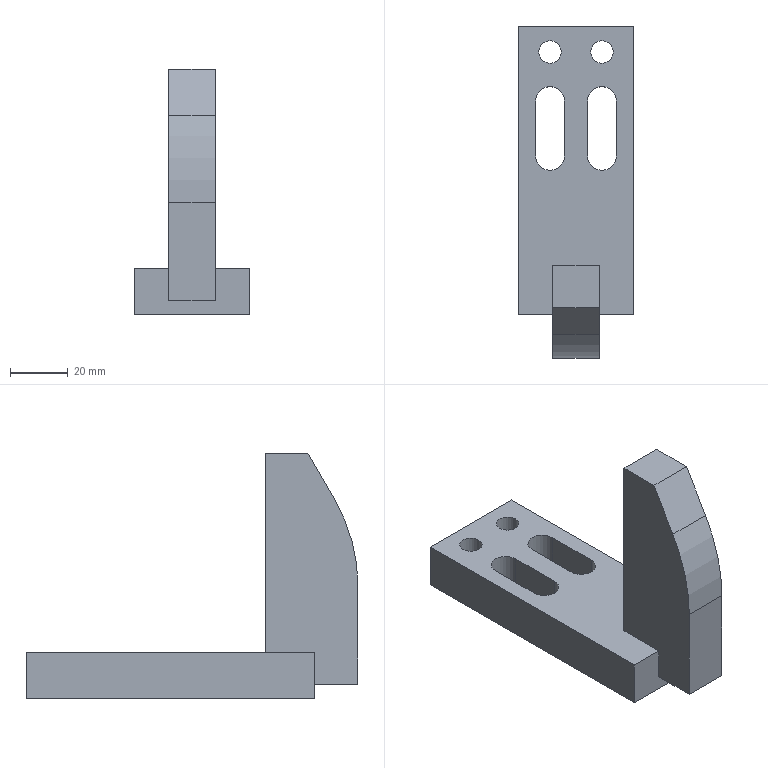Part | NX | features solid 2 | 1 solid | 24 faces | box 40 x 115 x 85 mm | volume 87334 mm3 | plane 17 | cylinder 7 | commonest cylinder face diameters 10 x4 7.8 x2 120 x1
STEP:
#1=CARTESIAN_POINT('',(797.6,496.,-19.));
#2=VERTEX_POINT('',#1);
#3=CARTESIAN_POINT('',(801.5,496.,-19.));
#4=DIRECTION('',(0.,0.,-1.));
#5=DIRECTION('',(-1.,0.,0.));
#6=AXIS2_PLACEMENT_3D('',#3,#4,#5);
#7=CIRCLE('',#6,3.9);
#8=EDGE_CURVE('',#2,#2,#7,.T.);
#9=ORIENTED_EDGE('',*,*,#8,.T.);
#10=EDGE_LOOP('',(#9));
#11=FACE_BOUND('',#10,.T.);
#12=CARTESIAN_POINT('',(806.5,460.,-19.));
#13=VERTEX_POINT('',#12);
#14=CARTESIAN_POINT('',(796.5,460.,-19.));
#15=VERTEX_POINT('',#14);
#16=CARTESIAN_POINT('',(801.5,460.,-19.));
#17=DIRECTION('',(0.,0.,-1.));
#18=DIRECTION('',(-1.,0.,0.));
#19=AXIS2_PLACEMENT_3D('',#16,#17,#18);
#20=CIRCLE('',#19,5.);
#21=EDGE_CURVE('',#13,#15,#20,.T.);
#22=ORIENTED_EDGE('',*,*,#21,.T.);
#23=CARTESIAN_POINT('',(796.5,479.,-19.));
#24=VERTEX_POINT('',#23);
#25=CARTESIAN_POINT('',(796.5,535.,-19.));
#26=DIRECTION('',(0.,-1.,0.));
#27=VECTOR('',#26,1000.);
#28=LINE('',#25,#27);
#29=EDGE_CURVE('',#24,#15,#28,.T.);
#30=ORIENTED_EDGE('',*,*,#29,.F.);
#31=CARTESIAN_POINT('',(806.5,479.,-19.));
#32=VERTEX_POINT('',#31);
#33=CARTESIAN_POINT('',(801.5,479.,-19.));
#34=DIRECTION('',(0.,0.,-1.));
#35=DIRECTION('',(-1.,0.,0.));
#36=AXIS2_PLACEMENT_3D('',#33,#34,#35);
#37=CIRCLE('',#36,5.);
#38=EDGE_CURVE('',#24,#32,#37,.T.);
#39=ORIENTED_EDGE('',*,*,#38,.T.);
#40=CARTESIAN_POINT('',(806.5,535.,-19.));
#41=DIRECTION('',(0.,1.,0.));
#42=VECTOR('',#41,1000.);
#43=LINE('',#40,#42);
#44=EDGE_CURVE('',#13,#32,#43,.T.);
#45=ORIENTED_EDGE('',*,*,#44,.F.);
#46=EDGE_LOOP('',(#22,#30,#39,#45));
#47=FACE_BOUND('',#46,.T.);
#48=CARTESIAN_POINT('',(779.6,496.,-19.));
#49=VERTEX_POINT('',#48);
#50=CARTESIAN_POINT('',(783.5,496.,-19.));
#51=DIRECTION('',(0.,0.,-1.));
#52=DIRECTION('',(-1.,0.,0.));
#53=AXIS2_PLACEMENT_3D('',#50,#51,#52);
#54=CIRCLE('',#53,3.9);
#55=EDGE_CURVE('',#49,#49,#54,.T.);
#56=ORIENTED_EDGE('',*,*,#55,.T.);
#57=EDGE_LOOP('',(#56));
#58=FACE_BOUND('',#57,.T.);
#59=CARTESIAN_POINT('',(812.5,405.,-19.));
#60=VERTEX_POINT('',#59);
#61=CARTESIAN_POINT('',(800.5,405.,-19.));
#62=VERTEX_POINT('',#61);
#63=CARTESIAN_POINT('',(804.5,405.,-19.));
#64=DIRECTION('',(-1.,0.,0.));
#65=VECTOR('',#64,1000.);
#66=LINE('',#63,#65);
#67=EDGE_CURVE('',#60,#62,#66,.T.);
#68=ORIENTED_EDGE('',*,*,#67,.F.);
#69=CARTESIAN_POINT('',(812.5,505.,-19.));
#70=VERTEX_POINT('',#69);
#71=CARTESIAN_POINT('',(812.5,505.,-19.));
#72=DIRECTION('',(0.,-1.,0.));
#73=VECTOR('',#72,1000.);
#74=LINE('',#71,#73);
#75=EDGE_CURVE('',#70,#60,#74,.T.);
#76=ORIENTED_EDGE('',*,*,#75,.F.);
#77=CARTESIAN_POINT('',(772.5,505.,-19.));
#78=VERTEX_POINT('',#77);
#79=CARTESIAN_POINT('',(804.5,505.,-19.));
#80=DIRECTION('',(1.,0.,0.));
#81=VECTOR('',#80,1000.);
#82=LINE('',#79,#81);
#83=EDGE_CURVE('',#78,#70,#82,.T.);
#84=ORIENTED_EDGE('',*,*,#83,.F.);
#85=CARTESIAN_POINT('',(772.5,405.,-19.));
#86=VERTEX_POINT('',#85);
#87=CARTESIAN_POINT('',(772.5,405.,-19.));
#88=DIRECTION('',(0.,1.,0.));
#89=VECTOR('',#88,1000.);
#90=LINE('',#87,#89);
#91=EDGE_CURVE('',#86,#78,#90,.T.);
#92=ORIENTED_EDGE('',*,*,#91,.F.);
#93=CARTESIAN_POINT('',(784.5,405.,-19.));
#94=VERTEX_POINT('',#93);
#95=CARTESIAN_POINT('',(804.5,405.,-19.));
#96=DIRECTION('',(-1.,0.,0.));
#97=VECTOR('',#96,1000.);
#98=LINE('',#95,#97);
#99=EDGE_CURVE('',#94,#86,#98,.T.);
#100=ORIENTED_EDGE('',*,*,#99,.F.);
#101=CARTESIAN_POINT('',(784.5,422.,-19.));
#102=VERTEX_POINT('',#101);
#103=CARTESIAN_POINT('',(784.5,505.,-19.));
#104=DIRECTION('',(0.,1.,0.));
#105=VECTOR('',#104,1000.);
#106=LINE('',#103,#105);
#107=EDGE_CURVE('',#94,#102,#106,.T.);
#108=ORIENTED_EDGE('',*,*,#107,.T.);
#109=CARTESIAN_POINT('',(800.5,422.,-19.));
#110=VERTEX_POINT('',#109);
#111=CARTESIAN_POINT('',(804.5,422.,-19.));
#112=DIRECTION('',(1.,0.,0.));
#113=VECTOR('',#112,1000.);
#114=LINE('',#111,#113);
#115=EDGE_CURVE('',#102,#110,#114,.T.);
#116=ORIENTED_EDGE('',*,*,#115,.T.);
#117=CARTESIAN_POINT('',(800.5,505.,-19.));
#118=DIRECTION('',(0.,1.,0.));
#119=VECTOR('',#118,1000.);
#120=LINE('',#117,#119);
#121=EDGE_CURVE('',#62,#110,#120,.T.);
#122=ORIENTED_EDGE('',*,*,#121,.F.);
#123=EDGE_LOOP('',(#68,#76,#84,#92,#100,#108,#116,#122));
#124=FACE_BOUND('',#123,.T.);
#125=CARTESIAN_POINT('',(778.5,479.,-19.));
#126=VERTEX_POINT('',#125);
#127=CARTESIAN_POINT('',(788.5,479.,-19.));
#128=VERTEX_POINT('',#127);
#129=CARTESIAN_POINT('',(783.5,479.,-19.));
#130=DIRECTION('',(0.,0.,-1.));
#131=DIRECTION('',(-1.,0.,0.));
#132=AXIS2_PLACEMENT_3D('',#129,#130,#131);
#133=CIRCLE('',#132,5.);
#134=EDGE_CURVE('',#126,#128,#133,.T.);
#135=ORIENTED_EDGE('',*,*,#134,.T.);
#136=CARTESIAN_POINT('',(788.5,460.,-19.));
#137=VERTEX_POINT('',#136);
#138=CARTESIAN_POINT('',(788.5,535.,-19.));
#139=DIRECTION('',(0.,1.,0.));
#140=VECTOR('',#139,1000.);
#141=LINE('',#138,#140);
#142=EDGE_CURVE('',#137,#128,#141,.T.);
#143=ORIENTED_EDGE('',*,*,#142,.F.);
#144=CARTESIAN_POINT('',(778.5,460.,-19.));
#145=VERTEX_POINT('',#144);
#146=CARTESIAN_POINT('',(783.5,460.,-19.));
#147=DIRECTION('',(0.,0.,-1.));
#148=DIRECTION('',(-1.,0.,0.));
#149=AXIS2_PLACEMENT_3D('',#146,#147,#148);
#150=CIRCLE('',#149,5.);
#151=EDGE_CURVE('',#137,#145,#150,.T.);
#152=ORIENTED_EDGE('',*,*,#151,.T.);
#153=CARTESIAN_POINT('',(778.5,535.,-19.));
#154=DIRECTION('',(0.,-1.,0.));
#155=VECTOR('',#154,1000.);
#156=LINE('',#153,#155);
#157=EDGE_CURVE('',#126,#145,#156,.T.);
#158=ORIENTED_EDGE('',*,*,#157,.F.);
#159=EDGE_LOOP('',(#135,#143,#152,#158));
#160=FACE_BOUND('',#159,.T.);
#161=CARTESIAN_POINT('',(804.5,505.,-19.));
#162=DIRECTION('',(0.,0.,1.));
#163=DIRECTION('',(0.,1.,0.));
#164=AXIS2_PLACEMENT_3D('',#161,#162,#163);
#165=PLANE('',#164);
#166=ADVANCED_FACE('',(#11,#47,#58,#124,#160),#165,.T.);
#167=CARTESIAN_POINT('',(797.6,496.,-35.));
#168=VERTEX_POINT('',#167);
#169=CARTESIAN_POINT('',(801.5,496.,-35.));
#170=DIRECTION('',(0.,0.,-1.));
#171=DIRECTION('',(-1.,0.,0.));
#172=AXIS2_PLACEMENT_3D('',#169,#170,#171);
#173=CIRCLE('',#172,3.9);
#174=EDGE_CURVE('',#168,#168,#173,.T.);
#175=ORIENTED_EDGE('',*,*,#174,.F.);
#176=EDGE_LOOP('',(#175));
#177=FACE_BOUND('',#176,.T.);
#178=CARTESIAN_POINT('',(806.5,460.,-35.));
#179=VERTEX_POINT('',#178);
#180=CARTESIAN_POINT('',(806.5,479.,-35.));
#181=VERTEX_POINT('',#180);
#182=CARTESIAN_POINT('',(806.5,535.,-35.));
#183=DIRECTION('',(0.,1.,0.));
#184=VECTOR('',#183,1000.);
#185=LINE('',#182,#184);
#186=EDGE_CURVE('',#179,#181,#185,.T.);
#187=ORIENTED_EDGE('',*,*,#186,.T.);
#188=CARTESIAN_POINT('',(796.5,479.,-35.));
#189=VERTEX_POINT('',#188);
#190=CARTESIAN_POINT('',(801.5,479.,-35.));
#191=DIRECTION('',(0.,0.,-1.));
#192=DIRECTION('',(-1.,0.,0.));
#193=AXIS2_PLACEMENT_3D('',#190,#191,#192);
#194=CIRCLE('',#193,5.);
#195=EDGE_CURVE('',#189,#181,#194,.T.);
#196=ORIENTED_EDGE('',*,*,#195,.F.);
#197=CARTESIAN_POINT('',(796.5,460.,-35.));
#198=VERTEX_POINT('',#197);
#199=CARTESIAN_POINT('',(796.5,535.,-35.));
#200=DIRECTION('',(0.,-1.,0.));
#201=VECTOR('',#200,1000.);
#202=LINE('',#199,#201);
#203=EDGE_CURVE('',#189,#198,#202,.T.);
#204=ORIENTED_EDGE('',*,*,#203,.T.);
#205=CARTESIAN_POINT('',(801.5,460.,-35.));
#206=DIRECTION('',(0.,0.,-1.));
#207=DIRECTION('',(-1.,0.,0.));
#208=AXIS2_PLACEMENT_3D('',#205,#206,#207);
#209=CIRCLE('',#208,5.);
#210=EDGE_CURVE('',#179,#198,#209,.T.);
#211=ORIENTED_EDGE('',*,*,#210,.F.);
#212=EDGE_LOOP('',(#187,#196,#204,#211));
#213=FACE_BOUND('',#212,.T.);
#214=CARTESIAN_POINT('',(779.6,496.,-35.));
#215=VERTEX_POINT('',#214);
#216=CARTESIAN_POINT('',(783.5,496.,-35.));
#217=DIRECTION('',(0.,0.,-1.));
#218=DIRECTION('',(-1.,0.,0.));
#219=AXIS2_PLACEMENT_3D('',#216,#217,#218);
#220=CIRCLE('',#219,3.9);
#221=EDGE_CURVE('',#215,#215,#220,.T.);
#222=ORIENTED_EDGE('',*,*,#221,.F.);
#223=EDGE_LOOP('',(#222));
#224=FACE_BOUND('',#223,.T.);
#225=CARTESIAN_POINT('',(772.5,505.,-35.));
#226=VERTEX_POINT('',#225);
#227=CARTESIAN_POINT('',(812.5,505.,-35.));
#228=VERTEX_POINT('',#227);
#229=CARTESIAN_POINT('',(804.5,505.,-35.));
#230=DIRECTION('',(1.,0.,0.));
#231=VECTOR('',#230,1000.);
#232=LINE('',#229,#231);
#233=EDGE_CURVE('',#226,#228,#232,.T.);
#234=ORIENTED_EDGE('',*,*,#233,.T.);
#235=CARTESIAN_POINT('',(812.5,405.,-35.));
#236=VERTEX_POINT('',#235);
#237=CARTESIAN_POINT('',(812.5,505.,-35.));
#238=DIRECTION('',(0.,-1.,0.));
#239=VECTOR('',#238,1000.);
#240=LINE('',#237,#239);
#241=EDGE_CURVE('',#228,#236,#240,.T.);
#242=ORIENTED_EDGE('',*,*,#241,.T.);
#243=CARTESIAN_POINT('',(772.5,405.,-35.));
#244=VERTEX_POINT('',#243);
#245=CARTESIAN_POINT('',(804.5,405.,-35.));
#246=DIRECTION('',(-1.,0.,0.));
#247=VECTOR('',#246,1000.);
#248=LINE('',#245,#247);
#249=EDGE_CURVE('',#236,#244,#248,.T.);
#250=ORIENTED_EDGE('',*,*,#249,.T.);
#251=CARTESIAN_POINT('',(772.5,405.,-35.));
#252=DIRECTION('',(0.,1.,0.));
#253=VECTOR('',#252,1000.);
#254=LINE('',#251,#253);
#255=EDGE_CURVE('',#244,#226,#254,.T.);
#256=ORIENTED_EDGE('',*,*,#255,.T.);
#257=EDGE_LOOP('',(#234,#242,#250,#256));
#258=FACE_BOUND('',#257,.T.);
#259=CARTESIAN_POINT('',(778.5,479.,-35.));
#260=VERTEX_POINT('',#259);
#261=CARTESIAN_POINT('',(778.5,460.,-35.));
#262=VERTEX_POINT('',#261);
#263=CARTESIAN_POINT('',(778.5,535.,-35.));
#264=DIRECTION('',(0.,-1.,0.));
#265=VECTOR('',#264,1000.);
#266=LINE('',#263,#265);
#267=EDGE_CURVE('',#260,#262,#266,.T.);
#268=ORIENTED_EDGE('',*,*,#267,.T.);
#269=CARTESIAN_POINT('',(788.5,460.,-35.));
#270=VERTEX_POINT('',#269);
#271=CARTESIAN_POINT('',(783.5,460.,-35.));
#272=DIRECTION('',(0.,0.,-1.));
#273=DIRECTION('',(-1.,0.,0.));
#274=AXIS2_PLACEMENT_3D('',#271,#272,#273);
#275=CIRCLE('',#274,5.);
#276=EDGE_CURVE('',#270,#262,#275,.T.);
#277=ORIENTED_EDGE('',*,*,#276,.F.);
#278=CARTESIAN_POINT('',(788.5,479.,-35.));
#279=VERTEX_POINT('',#278);
#280=CARTESIAN_POINT('',(788.5,535.,-35.));
#281=DIRECTION('',(0.,1.,0.));
#282=VECTOR('',#281,1000.);
#283=LINE('',#280,#282);
#284=EDGE_CURVE('',#270,#279,#283,.T.);
#285=ORIENTED_EDGE('',*,*,#284,.T.);
#286=CARTESIAN_POINT('',(783.5,479.,-35.));
#287=DIRECTION('',(0.,0.,-1.));
#288=DIRECTION('',(-1.,0.,0.));
#289=AXIS2_PLACEMENT_3D('',#286,#287,#288);
#290=CIRCLE('',#289,5.);
#291=EDGE_CURVE('',#260,#279,#290,.T.);
#292=ORIENTED_EDGE('',*,*,#291,.F.);
#293=EDGE_LOOP('',(#268,#277,#285,#292));
#294=FACE_BOUND('',#293,.T.);
#295=CARTESIAN_POINT('',(804.5,505.,-35.));
#296=DIRECTION('',(0.,0.,1.));
#297=DIRECTION('',(0.,1.,0.));
#298=AXIS2_PLACEMENT_3D('',#295,#296,#297);
#299=PLANE('',#298);
#300=ADVANCED_FACE('',(#177,#213,#224,#258,#294),#299,.F.);
#301=CARTESIAN_POINT('',(800.5,405.,-30.));
#302=VERTEX_POINT('',#301);
#303=CARTESIAN_POINT('',(800.5,405.,-19.));
#304=DIRECTION('',(0.,0.,-1.));
#305=VECTOR('',#304,1000.);
#306=LINE('',#303,#305);
#307=EDGE_CURVE('',#62,#302,#306,.T.);
#308=ORIENTED_EDGE('',*,*,#307,.T.);
#309=CARTESIAN_POINT('',(784.5,405.,-30.));
#310=VERTEX_POINT('',#309);
#311=CARTESIAN_POINT('',(804.5,405.,-30.));
#312=DIRECTION('',(1.,0.,0.));
#313=VECTOR('',#312,1000.);
#314=LINE('',#311,#313);
#315=EDGE_CURVE('',#310,#302,#314,.T.);
#316=ORIENTED_EDGE('',*,*,#315,.F.);
#317=CARTESIAN_POINT('',(784.5,405.,-19.));
#318=DIRECTION('',(0.,0.,-1.));
#319=VECTOR('',#318,1000.);
#320=LINE('',#317,#319);
#321=EDGE_CURVE('',#94,#310,#320,.T.);
#322=ORIENTED_EDGE('',*,*,#321,.F.);
#323=ORIENTED_EDGE('',*,*,#99,.T.);
#324=CARTESIAN_POINT('',(772.5,405.,-19.));
#325=DIRECTION('',(0.,0.,-1.));
#326=VECTOR('',#325,1000.);
#327=LINE('',#324,#326);
#328=EDGE_CURVE('',#86,#244,#327,.T.);
#329=ORIENTED_EDGE('',*,*,#328,.T.);
#330=ORIENTED_EDGE('',*,*,#249,.F.);
#331=CARTESIAN_POINT('',(812.5,405.,-19.));
#332=DIRECTION('',(0.,0.,-1.));
#333=VECTOR('',#332,1000.);
#334=LINE('',#331,#333);
#335=EDGE_CURVE('',#60,#236,#334,.T.);
#336=ORIENTED_EDGE('',*,*,#335,.F.);
#337=ORIENTED_EDGE('',*,*,#67,.T.);
#338=EDGE_LOOP('',(#308,#316,#322,#323,#329,#330,#336,#337));
#339=FACE_BOUND('',#338,.T.);
#340=CARTESIAN_POINT('',(804.5,405.,-19.));
#341=DIRECTION('',(0.,1.,0.));
#342=DIRECTION('',(0.,0.,-1.));
#343=AXIS2_PLACEMENT_3D('',#340,#341,#342);
#344=PLANE('',#343);
#345=ADVANCED_FACE('',(#339),#344,.F.);
#346=ORIENTED_EDGE('',*,*,#233,.F.);
#347=CARTESIAN_POINT('',(772.5,505.,-19.));
#348=DIRECTION('',(0.,0.,-1.));
#349=VECTOR('',#348,1000.);
#350=LINE('',#347,#349);
#351=EDGE_CURVE('',#78,#226,#350,.T.);
#352=ORIENTED_EDGE('',*,*,#351,.F.);
#353=ORIENTED_EDGE('',*,*,#83,.T.);
#354=CARTESIAN_POINT('',(812.5,505.,-19.));
#355=DIRECTION('',(0.,0.,-1.));
#356=VECTOR('',#355,1000.);
#357=LINE('',#354,#356);
#358=EDGE_CURVE('',#70,#228,#357,.T.);
#359=ORIENTED_EDGE('',*,*,#358,.T.);
#360=EDGE_LOOP('',(#346,#352,#353,#359));
#361=FACE_BOUND('',#360,.T.);
#362=CARTESIAN_POINT('',(780.5,505.,-19.));
#363=DIRECTION('',(0.,-1.,0.));
#364=DIRECTION('',(0.,0.,1.));
#365=AXIS2_PLACEMENT_3D('',#362,#363,#364);
#366=PLANE('',#365);
#367=ADVANCED_FACE('',(#361),#366,.F.);
#368=ORIENTED_EDGE('',*,*,#241,.F.);
#369=ORIENTED_EDGE('',*,*,#358,.F.);
#370=ORIENTED_EDGE('',*,*,#75,.T.);
#371=ORIENTED_EDGE('',*,*,#335,.T.);
#372=EDGE_LOOP('',(#368,#369,#370,#371));
#373=FACE_BOUND('',#372,.T.);
#374=CARTESIAN_POINT('',(812.5,505.,-19.));
#375=DIRECTION('',(-1.,0.,0.));
#376=DIRECTION('',(0.,0.,-1.));
#377=AXIS2_PLACEMENT_3D('',#374,#375,#376);
#378=PLANE('',#377);
#379=ADVANCED_FACE('',(#373),#378,.F.);
#380=ORIENTED_EDGE('',*,*,#255,.F.);
#381=ORIENTED_EDGE('',*,*,#328,.F.);
#382=ORIENTED_EDGE('',*,*,#91,.T.);
#383=ORIENTED_EDGE('',*,*,#351,.T.);
#384=EDGE_LOOP('',(#380,#381,#382,#383));
#385=FACE_BOUND('',#384,.T.);
#386=CARTESIAN_POINT('',(772.5,405.,-19.));
#387=DIRECTION('',(1.,0.,0.));
#388=DIRECTION('',(0.,0.,1.));
#389=AXIS2_PLACEMENT_3D('',#386,#387,#388);
#390=PLANE('',#389);
#391=ADVANCED_FACE('',(#385),#390,.F.);
#392=ORIENTED_EDGE('',*,*,#315,.T.);
#393=CARTESIAN_POINT('',(800.5,390.,-30.));
#394=VERTEX_POINT('',#393);
#395=CARTESIAN_POINT('',(800.5,390.,-30.));
#396=DIRECTION('',(0.,1.,0.));
#397=VECTOR('',#396,1000.);
#398=LINE('',#395,#397);
#399=EDGE_CURVE('',#394,#302,#398,.T.);
#400=ORIENTED_EDGE('',*,*,#399,.F.);
#401=CARTESIAN_POINT('',(784.5,390.,-30.));
#402=VERTEX_POINT('',#401);
#403=CARTESIAN_POINT('',(800.5,390.,-30.));
#404=DIRECTION('',(-1.,0.,0.));
#405=VECTOR('',#404,1000.);
#406=LINE('',#403,#405);
#407=EDGE_CURVE('',#394,#402,#406,.T.);
#408=ORIENTED_EDGE('',*,*,#407,.T.);
#409=CARTESIAN_POINT('',(784.5,390.,-30.));
#410=DIRECTION('',(0.,1.,0.));
#411=VECTOR('',#410,1000.);
#412=LINE('',#409,#411);
#413=EDGE_CURVE('',#402,#310,#412,.T.);
#414=ORIENTED_EDGE('',*,*,#413,.T.);
#415=EDGE_LOOP('',(#392,#400,#408,#414));
#416=FACE_BOUND('',#415,.T.);
#417=CARTESIAN_POINT('',(800.5,390.,-30.));
#418=DIRECTION('',(0.,0.,-1.));
#419=DIRECTION('',(0.,-1.,0.));
#420=AXIS2_PLACEMENT_3D('',#417,#418,#419);
#421=PLANE('',#420);
#422=ADVANCED_FACE('',(#416),#421,.T.);
#423=ORIENTED_EDGE('',*,*,#121,.T.);
#424=CARTESIAN_POINT('',(800.5,422.,50.));
#425=VERTEX_POINT('',#424);
#426=CARTESIAN_POINT('',(800.5,422.,-30.));
#427=DIRECTION('',(0.,0.,1.));
#428=VECTOR('',#427,1000.);
#429=LINE('',#426,#428);
#430=EDGE_CURVE('',#110,#425,#429,.T.);
#431=ORIENTED_EDGE('',*,*,#430,.T.);
#432=CARTESIAN_POINT('',(800.5,407.322,50.));
#433=VERTEX_POINT('',#432);
#434=CARTESIAN_POINT('',(800.5,422.,50.));
#435=DIRECTION('',(0.,-1.,0.));
#436=VECTOR('',#435,1000.);
#437=LINE('',#434,#436);
#438=EDGE_CURVE('',#425,#433,#437,.T.);
#439=ORIENTED_EDGE('',*,*,#438,.T.);
#440=CARTESIAN_POINT('',(800.5,398.04,33.924));
#441=VERTEX_POINT('',#440);
#442=CARTESIAN_POINT('',(800.5,407.322,50.));
#443=DIRECTION('',(0.,-0.5,-0.866));
#444=VECTOR('',#443,1000.);
#445=LINE('',#442,#444);
#446=EDGE_CURVE('',#433,#441,#445,.T.);
#447=ORIENTED_EDGE('',*,*,#446,.T.);
#448=CARTESIAN_POINT('',(800.5,390.,3.922));
#449=VERTEX_POINT('',#448);
#450=CARTESIAN_POINT('',(800.5,450.,3.922));
#451=DIRECTION('',(1.,0.,0.));
#452=DIRECTION('',(0.,0.,-1.));
#453=AXIS2_PLACEMENT_3D('',#450,#451,#452);
#454=CIRCLE('',#453,60.);
#455=EDGE_CURVE('',#449,#441,#454,.F.);
#456=ORIENTED_EDGE('',*,*,#455,.F.);
#457=CARTESIAN_POINT('',(800.5,390.,15.));
#458=DIRECTION('',(0.,0.,-1.));
#459=VECTOR('',#458,1000.);
#460=LINE('',#457,#459);
#461=EDGE_CURVE('',#449,#394,#460,.T.);
#462=ORIENTED_EDGE('',*,*,#461,.T.);
#463=ORIENTED_EDGE('',*,*,#399,.T.);
#464=ORIENTED_EDGE('',*,*,#307,.F.);
#465=EDGE_LOOP('',(#423,#431,#439,#447,#456,#462,#463,#464));
#466=FACE_BOUND('',#465,.T.);
#467=CARTESIAN_POINT('',(800.5,422.,45.));
#468=DIRECTION('',(-1.,0.,0.));
#469=DIRECTION('',(0.,0.,-1.));
#470=AXIS2_PLACEMENT_3D('',#467,#468,#469);
#471=PLANE('',#470);
#472=ADVANCED_FACE('',(#466),#471,.F.);
#473=ORIENTED_EDGE('',*,*,#321,.T.);
#474=ORIENTED_EDGE('',*,*,#413,.F.);
#475=CARTESIAN_POINT('',(784.5,390.,3.922));
#476=VERTEX_POINT('',#475);
#477=CARTESIAN_POINT('',(784.5,390.,15.));
#478=DIRECTION('',(0.,0.,-1.));
#479=VECTOR('',#478,1000.);
#480=LINE('',#477,#479);
#481=EDGE_CURVE('',#476,#402,#480,.T.);
#482=ORIENTED_EDGE('',*,*,#481,.F.);
#483=CARTESIAN_POINT('',(784.5,398.04,33.924));
#484=VERTEX_POINT('',#483);
#485=CARTESIAN_POINT('',(784.5,450.,3.922));
#486=DIRECTION('',(1.,0.,0.));
#487=DIRECTION('',(0.,0.,-1.));
#488=AXIS2_PLACEMENT_3D('',#485,#486,#487);
#489=CIRCLE('',#488,60.);
#490=EDGE_CURVE('',#484,#476,#489,.T.);
#491=ORIENTED_EDGE('',*,*,#490,.F.);
#492=CARTESIAN_POINT('',(784.5,407.322,50.));
#493=VERTEX_POINT('',#492);
#494=CARTESIAN_POINT('',(784.5,407.322,50.));
#495=DIRECTION('',(0.,-0.5,-0.866));
#496=VECTOR('',#495,1000.);
#497=LINE('',#494,#496);
#498=EDGE_CURVE('',#493,#484,#497,.T.);
#499=ORIENTED_EDGE('',*,*,#498,.F.);
#500=CARTESIAN_POINT('',(784.5,422.,50.));
#501=VERTEX_POINT('',#500);
#502=CARTESIAN_POINT('',(784.5,422.,50.));
#503=DIRECTION('',(0.,-1.,0.));
#504=VECTOR('',#503,1000.);
#505=LINE('',#502,#504);
#506=EDGE_CURVE('',#501,#493,#505,.T.);
#507=ORIENTED_EDGE('',*,*,#506,.F.);
#508=CARTESIAN_POINT('',(784.5,422.,-30.));
#509=DIRECTION('',(0.,0.,1.));
#510=VECTOR('',#509,1000.);
#511=LINE('',#508,#510);
#512=EDGE_CURVE('',#102,#501,#511,.T.);
#513=ORIENTED_EDGE('',*,*,#512,.F.);
#514=ORIENTED_EDGE('',*,*,#107,.F.);
#515=EDGE_LOOP('',(#473,#474,#482,#491,#499,#507,#513,#514));
#516=FACE_BOUND('',#515,.T.);
#517=CARTESIAN_POINT('',(784.5,422.,45.));
#518=DIRECTION('',(-1.,0.,0.));
#519=DIRECTION('',(0.,0.,-1.));
#520=AXIS2_PLACEMENT_3D('',#517,#518,#519);
#521=PLANE('',#520);
#522=ADVANCED_FACE('',(#516),#521,.T.);
#523=ORIENTED_EDGE('',*,*,#512,.T.);
#524=CARTESIAN_POINT('',(800.5,422.,50.));
#525=DIRECTION('',(-1.,0.,0.));
#526=VECTOR('',#525,1000.);
#527=LINE('',#524,#526);
#528=EDGE_CURVE('',#425,#501,#527,.T.);
#529=ORIENTED_EDGE('',*,*,#528,.F.);
#530=ORIENTED_EDGE('',*,*,#430,.F.);
#531=ORIENTED_EDGE('',*,*,#115,.F.);
#532=EDGE_LOOP('',(#523,#529,#530,#531));
#533=FACE_BOUND('',#532,.T.);
#534=CARTESIAN_POINT('',(800.5,422.,-30.));
#535=DIRECTION('',(0.,1.,0.));
#536=DIRECTION('',(0.,0.,-1.));
#537=AXIS2_PLACEMENT_3D('',#534,#535,#536);
#538=PLANE('',#537);
#539=ADVANCED_FACE('',(#533),#538,.T.);
#540=CARTESIAN_POINT('',(800.5,407.322,50.));
#541=DIRECTION('',(-1.,0.,0.));
#542=VECTOR('',#541,1000.);
#543=LINE('',#540,#542);
#544=EDGE_CURVE('',#433,#493,#543,.T.);
#545=ORIENTED_EDGE('',*,*,#544,.F.);
#546=ORIENTED_EDGE('',*,*,#438,.F.);
#547=ORIENTED_EDGE('',*,*,#528,.T.);
#548=ORIENTED_EDGE('',*,*,#506,.T.);
#549=EDGE_LOOP('',(#545,#546,#547,#548));
#550=FACE_BOUND('',#549,.T.);
#551=CARTESIAN_POINT('',(800.5,422.,50.));
#552=DIRECTION('',(0.,0.,1.));
#553=DIRECTION('',(0.,1.,0.));
#554=AXIS2_PLACEMENT_3D('',#551,#552,#553);
#555=PLANE('',#554);
#556=ADVANCED_FACE('',(#550),#555,.T.);
#557=ORIENTED_EDGE('',*,*,#446,.F.);
#558=ORIENTED_EDGE('',*,*,#544,.T.);
#559=ORIENTED_EDGE('',*,*,#498,.T.);
#560=CARTESIAN_POINT('',(800.5,398.04,33.924));
#561=DIRECTION('',(-1.,0.,0.));
#562=VECTOR('',#561,1000.);
#563=LINE('',#560,#562);
#564=EDGE_CURVE('',#441,#484,#563,.T.);
#565=ORIENTED_EDGE('',*,*,#564,.F.);
#566=EDGE_LOOP('',(#557,#558,#559,#565));
#567=FACE_BOUND('',#566,.T.);
#568=CARTESIAN_POINT('',(800.5,407.322,50.));
#569=DIRECTION('',(0.,-0.866,0.5));
#570=DIRECTION('',(0.,0.5,0.866));
#571=AXIS2_PLACEMENT_3D('',#568,#569,#570);
#572=PLANE('',#571);
#573=ADVANCED_FACE('',(#567),#572,.T.);
#574=ORIENTED_EDGE('',*,*,#481,.T.);
#575=ORIENTED_EDGE('',*,*,#407,.F.);
#576=ORIENTED_EDGE('',*,*,#461,.F.);
#577=CARTESIAN_POINT('',(800.5,390.,3.922));
#578=DIRECTION('',(-1.,0.,0.));
#579=VECTOR('',#578,1000.);
#580=LINE('',#577,#579);
#581=EDGE_CURVE('',#476,#449,#580,.F.);
#582=ORIENTED_EDGE('',*,*,#581,.F.);
#583=EDGE_LOOP('',(#574,#575,#576,#582));
#584=FACE_BOUND('',#583,.T.);
#585=CARTESIAN_POINT('',(800.5,390.,15.));
#586=DIRECTION('',(0.,-1.,0.));
#587=DIRECTION('',(0.,0.,1.));
#588=AXIS2_PLACEMENT_3D('',#585,#586,#587);
#589=PLANE('',#588);
#590=ADVANCED_FACE('',(#584),#589,.T.);
#591=ORIENTED_EDGE('',*,*,#455,.T.);
#592=ORIENTED_EDGE('',*,*,#564,.T.);
#593=ORIENTED_EDGE('',*,*,#490,.T.);
#594=ORIENTED_EDGE('',*,*,#581,.T.);
#595=EDGE_LOOP('',(#591,#592,#593,#594));
#596=FACE_BOUND('',#595,.T.);
#597=CARTESIAN_POINT('',(800.5,450.,3.922));
#598=DIRECTION('',(-1.,0.,0.));
#599=DIRECTION('',(0.,0.,-1.));
#600=AXIS2_PLACEMENT_3D('',#597,#598,#599);
#601=CYLINDRICAL_SURFACE('',#600,60.);
#602=ADVANCED_FACE('',(#596),#601,.T.);
#603=CARTESIAN_POINT('',(778.5,479.,16.));
#604=DIRECTION('',(0.,0.,-1.));
#605=VECTOR('',#604,1000.);
#606=LINE('',#603,#605);
#607=EDGE_CURVE('',#126,#260,#606,.T.);
#608=ORIENTED_EDGE('',*,*,#607,.F.);
#609=ORIENTED_EDGE('',*,*,#157,.T.);
#610=CARTESIAN_POINT('',(778.5,460.,16.));
#611=DIRECTION('',(0.,0.,-1.));
#612=VECTOR('',#611,1000.);
#613=LINE('',#610,#612);
#614=EDGE_CURVE('',#145,#262,#613,.T.);
#615=ORIENTED_EDGE('',*,*,#614,.T.);
#616=ORIENTED_EDGE('',*,*,#267,.F.);
#617=EDGE_LOOP('',(#608,#609,#615,#616));
#618=FACE_BOUND('',#617,.T.);
#619=CARTESIAN_POINT('',(778.5,465.,16.));
#620=DIRECTION('',(1.,0.,0.));
#621=DIRECTION('',(0.,0.,1.));
#622=AXIS2_PLACEMENT_3D('',#619,#620,#621);
#623=PLANE('',#622);
#624=ADVANCED_FACE('',(#618),#623,.T.);
#625=ORIENTED_EDGE('',*,*,#134,.F.);
#626=ORIENTED_EDGE('',*,*,#607,.T.);
#627=ORIENTED_EDGE('',*,*,#291,.T.);
#628=CARTESIAN_POINT('',(788.5,479.,16.));
#629=DIRECTION('',(0.,0.,-1.));
#630=VECTOR('',#629,1000.);
#631=LINE('',#628,#630);
#632=EDGE_CURVE('',#128,#279,#631,.T.);
#633=ORIENTED_EDGE('',*,*,#632,.F.);
#634=EDGE_LOOP('',(#625,#626,#627,#633));
#635=FACE_BOUND('',#634,.T.);
#636=CARTESIAN_POINT('',(783.5,479.,16.));
#637=DIRECTION('',(0.,0.,-1.));
#638=DIRECTION('',(1.,0.,0.));
#639=AXIS2_PLACEMENT_3D('',#636,#637,#638);
#640=CYLINDRICAL_SURFACE('',#639,5.);
#641=ADVANCED_FACE('',(#635),#640,.F.);
#642=CARTESIAN_POINT('',(788.5,460.,16.));
#643=DIRECTION('',(0.,0.,-1.));
#644=VECTOR('',#643,1000.);
#645=LINE('',#642,#644);
#646=EDGE_CURVE('',#137,#270,#645,.T.);
#647=ORIENTED_EDGE('',*,*,#646,.F.);
#648=ORIENTED_EDGE('',*,*,#142,.T.);
#649=ORIENTED_EDGE('',*,*,#632,.T.);
#650=ORIENTED_EDGE('',*,*,#284,.F.);
#651=EDGE_LOOP('',(#647,#648,#649,#650));
#652=FACE_BOUND('',#651,.T.);
#653=CARTESIAN_POINT('',(788.5,484.,16.));
#654=DIRECTION('',(-1.,0.,0.));
#655=DIRECTION('',(0.,0.,-1.));
#656=AXIS2_PLACEMENT_3D('',#653,#654,#655);
#657=PLANE('',#656);
#658=ADVANCED_FACE('',(#652),#657,.T.);
#659=ORIENTED_EDGE('',*,*,#151,.F.);
#660=ORIENTED_EDGE('',*,*,#646,.T.);
#661=ORIENTED_EDGE('',*,*,#276,.T.);
#662=ORIENTED_EDGE('',*,*,#614,.F.);
#663=EDGE_LOOP('',(#659,#660,#661,#662));
#664=FACE_BOUND('',#663,.T.);
#665=CARTESIAN_POINT('',(783.5,460.,16.));
#666=DIRECTION('',(0.,0.,-1.));
#667=DIRECTION('',(1.,0.,0.));
#668=AXIS2_PLACEMENT_3D('',#665,#666,#667);
#669=CYLINDRICAL_SURFACE('',#668,5.);
#670=ADVANCED_FACE('',(#664),#669,.F.);
#671=ORIENTED_EDGE('',*,*,#55,.F.);
#672=EDGE_LOOP('',(#671));
#673=FACE_BOUND('',#672,.T.);
#674=ORIENTED_EDGE('',*,*,#221,.T.);
#675=EDGE_LOOP('',(#674));
#676=FACE_BOUND('',#675,.T.);
#677=CARTESIAN_POINT('',(783.5,496.,16.));
#678=DIRECTION('',(0.,0.,-1.));
#679=DIRECTION('',(1.,0.,0.));
#680=AXIS2_PLACEMENT_3D('',#677,#678,#679);
#681=CYLINDRICAL_SURFACE('',#680,3.9);
#682=ADVANCED_FACE('',(#673,#676),#681,.F.);
#683=ORIENTED_EDGE('',*,*,#21,.F.);
#684=CARTESIAN_POINT('',(806.5,460.,16.));
#685=DIRECTION('',(0.,0.,-1.));
#686=VECTOR('',#685,1000.);
#687=LINE('',#684,#686);
#688=EDGE_CURVE('',#13,#179,#687,.T.);
#689=ORIENTED_EDGE('',*,*,#688,.T.);
#690=ORIENTED_EDGE('',*,*,#210,.T.);
#691=CARTESIAN_POINT('',(796.5,460.,16.));
#692=DIRECTION('',(0.,0.,-1.));
#693=VECTOR('',#692,1000.);
#694=LINE('',#691,#693);
#695=EDGE_CURVE('',#15,#198,#694,.T.);
#696=ORIENTED_EDGE('',*,*,#695,.F.);
#697=EDGE_LOOP('',(#683,#689,#690,#696));
#698=FACE_BOUND('',#697,.T.);
#699=CARTESIAN_POINT('',(801.5,460.,16.));
#700=DIRECTION('',(0.,0.,-1.));
#701=DIRECTION('',(1.,0.,0.));
#702=AXIS2_PLACEMENT_3D('',#699,#700,#701);
#703=CYLINDRICAL_SURFACE('',#702,5.);
#704=ADVANCED_FACE('',(#698),#703,.F.);
#705=ORIENTED_EDGE('',*,*,#688,.F.);
#706=ORIENTED_EDGE('',*,*,#44,.T.);
#707=CARTESIAN_POINT('',(806.5,479.,16.));
#708=DIRECTION('',(0.,0.,-1.));
#709=VECTOR('',#708,1000.);
#710=LINE('',#707,#709);
#711=EDGE_CURVE('',#32,#181,#710,.T.);
#712=ORIENTED_EDGE('',*,*,#711,.T.);
#713=ORIENTED_EDGE('',*,*,#186,.F.);
#714=EDGE_LOOP('',(#705,#706,#712,#713));
#715=FACE_BOUND('',#714,.T.);
#716=CARTESIAN_POINT('',(806.5,484.,16.));
#717=DIRECTION('',(-1.,0.,0.));
#718=DIRECTION('',(0.,0.,-1.));
#719=AXIS2_PLACEMENT_3D('',#716,#717,#718);
#720=PLANE('',#719);
#721=ADVANCED_FACE('',(#715),#720,.T.);
#722=ORIENTED_EDGE('',*,*,#38,.F.);
#723=CARTESIAN_POINT('',(796.5,479.,16.));
#724=DIRECTION('',(0.,0.,-1.));
#725=VECTOR('',#724,1000.);
#726=LINE('',#723,#725);
#727=EDGE_CURVE('',#24,#189,#726,.T.);
#728=ORIENTED_EDGE('',*,*,#727,.T.);
#729=ORIENTED_EDGE('',*,*,#195,.T.);
#730=ORIENTED_EDGE('',*,*,#711,.F.);
#731=EDGE_LOOP('',(#722,#728,#729,#730));
#732=FACE_BOUND('',#731,.T.);
#733=CARTESIAN_POINT('',(801.5,479.,16.));
#734=DIRECTION('',(0.,0.,-1.));
#735=DIRECTION('',(1.,0.,0.));
#736=AXIS2_PLACEMENT_3D('',#733,#734,#735);
#737=CYLINDRICAL_SURFACE('',#736,5.);
#738=ADVANCED_FACE('',(#732),#737,.F.);
#739=ORIENTED_EDGE('',*,*,#727,.F.);
#740=ORIENTED_EDGE('',*,*,#29,.T.);
#741=ORIENTED_EDGE('',*,*,#695,.T.);
#742=ORIENTED_EDGE('',*,*,#203,.F.);
#743=EDGE_LOOP('',(#739,#740,#741,#742));
#744=FACE_BOUND('',#743,.T.);
#745=CARTESIAN_POINT('',(796.5,465.,16.));
#746=DIRECTION('',(1.,0.,0.));
#747=DIRECTION('',(0.,0.,1.));
#748=AXIS2_PLACEMENT_3D('',#745,#746,#747);
#749=PLANE('',#748);
#750=ADVANCED_FACE('',(#744),#749,.T.);
#751=ORIENTED_EDGE('',*,*,#8,.F.);
#752=EDGE_LOOP('',(#751));
#753=FACE_BOUND('',#752,.T.);
#754=ORIENTED_EDGE('',*,*,#174,.T.);
#755=EDGE_LOOP('',(#754));
#756=FACE_BOUND('',#755,.T.);
#757=CARTESIAN_POINT('',(801.5,496.,16.));
#758=DIRECTION('',(0.,0.,-1.));
#759=DIRECTION('',(1.,0.,0.));
#760=AXIS2_PLACEMENT_3D('',#757,#758,#759);
#761=CYLINDRICAL_SURFACE('',#760,3.9);
#762=ADVANCED_FACE('',(#753,#756),#761,.F.);
#763=CLOSED_SHELL('',(#166,#300,#345,#367,#379,#391,#422,#472,#522,#539,#556,#573,#590,#602,#624,#641,#658,#670,#682,#704,#721,#738,#750,#762));
#764=MANIFOLD_SOLID_BREP('',#763);
#765=(LENGTH_UNIT()NAMED_UNIT(*)SI_UNIT(.MILLI.,.METRE.));
#766=UNCERTAINTY_MEASURE_WITH_UNIT(LENGTH_MEASURE(0.00001),#765,'','');
#767=(NAMED_UNIT(*)PLANE_ANGLE_UNIT()SI_UNIT($,.RADIAN.));
#768=(NAMED_UNIT(*)SI_UNIT($,.STERADIAN.)SOLID_ANGLE_UNIT());
#769=(GEOMETRIC_REPRESENTATION_CONTEXT(3)GLOBAL_UNCERTAINTY_ASSIGNED_CONTEXT((#766))GLOBAL_UNIT_ASSIGNED_CONTEXT((#765,#767,#768))REPRESENTATION_CONTEXT('',''));
#770=ADVANCED_BREP_SHAPE_REPRESENTATION('',(#764),#769);